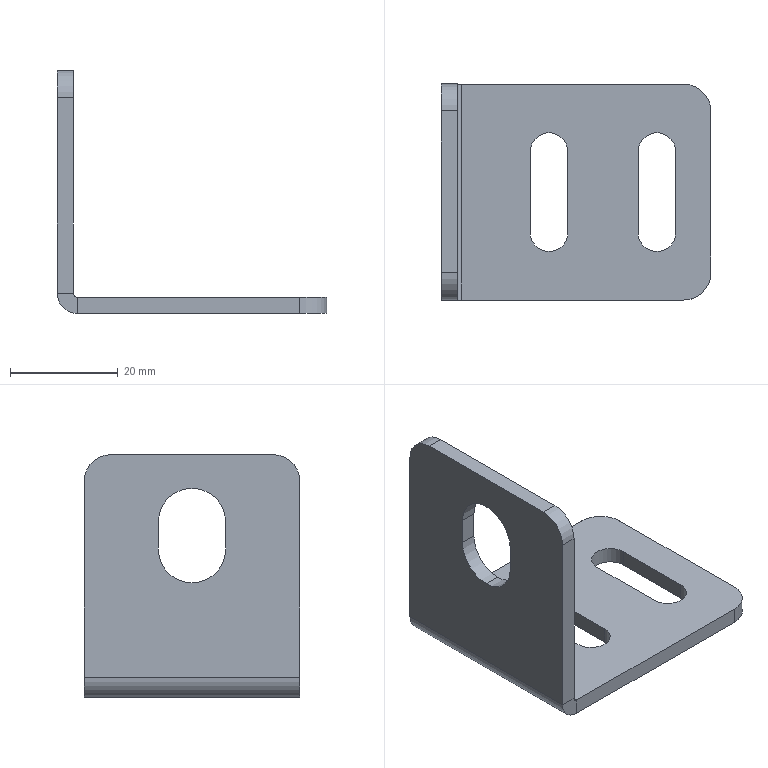Part | SolidWorks | features BaseBody 1 | 1 solid | 31 faces | box 50 x 40 x 45 mm | volume 9444 mm3 | plane 18 | cylinder 13 | commonest cylinder face diameters 7 x4 10 x4 12.5 x3 1.473 x1 7.473 x1
STEP:
#1=CARTESIAN_POINT('',(-25.,0.,18.25));
#2=VERTEX_POINT('',#1);
#3=CARTESIAN_POINT('',(-25.,6.25,24.5));
#4=VERTEX_POINT('',#3);
#5=CARTESIAN_POINT('',(-25.,0.,24.5));
#6=DIRECTION('',(1.,0.,0.));
#7=DIRECTION('',(0.,0.,-1.));
#8=AXIS2_PLACEMENT_3D('',#5,#6,#7);
#9=CIRCLE('',#8,6.25);
#10=EDGE_CURVE('',#2,#4,#9,.T.);
#11=ORIENTED_EDGE('',*,*,#10,.F.);
#12=CARTESIAN_POINT('',(-22.,0.,18.25));
#13=VERTEX_POINT('',#12);
#14=CARTESIAN_POINT('',(-32.,0.,18.25));
#15=DIRECTION('',(1.,0.,0.));
#16=VECTOR('',#15,1000.);
#17=LINE('',#14,#16);
#18=EDGE_CURVE('',#2,#13,#17,.T.);
#19=ORIENTED_EDGE('',*,*,#18,.T.);
#20=CARTESIAN_POINT('',(-22.,6.25,24.5));
#21=VERTEX_POINT('',#20);
#22=CARTESIAN_POINT('',(-22.,0.,24.5));
#23=DIRECTION('',(1.,0.,0.));
#24=DIRECTION('',(0.,0.,-1.));
#25=AXIS2_PLACEMENT_3D('',#22,#23,#24);
#26=CIRCLE('',#25,6.25);
#27=EDGE_CURVE('',#13,#21,#26,.T.);
#28=ORIENTED_EDGE('',*,*,#27,.T.);
#29=CARTESIAN_POINT('',(-32.,6.25,24.5));
#30=DIRECTION('',(1.,0.,0.));
#31=VECTOR('',#30,1000.);
#32=LINE('',#29,#31);
#33=EDGE_CURVE('',#4,#21,#32,.T.);
#34=ORIENTED_EDGE('',*,*,#33,.F.);
#35=EDGE_LOOP('',(#11,#19,#28,#34));
#36=FACE_OUTER_BOUND('',#35,.T.);
#37=CARTESIAN_POINT('',(-32.,0.,24.5));
#38=DIRECTION('',(1.,0.,0.));
#39=DIRECTION('',(0.,0.,-1.));
#40=AXIS2_PLACEMENT_3D('',#37,#38,#39);
#41=CYLINDRICAL_SURFACE('',#40,6.25);
#42=ADVANCED_FACE('',(#36),#41,.F.);
#43=CARTESIAN_POINT('',(-21.263,-20.,-3.));
#44=VERTEX_POINT('',#43);
#45=CARTESIAN_POINT('',(20.,-20.,-3.));
#46=VERTEX_POINT('',#45);
#47=CARTESIAN_POINT('',(-25.,-20.,-3.));
#48=DIRECTION('',(1.,0.,0.));
#49=VECTOR('',#48,1000.);
#50=LINE('',#47,#49);
#51=EDGE_CURVE('',#44,#46,#50,.T.);
#52=ORIENTED_EDGE('',*,*,#51,.T.);
#53=CARTESIAN_POINT('',(20.,-20.,0.));
#54=VERTEX_POINT('',#53);
#55=CARTESIAN_POINT('',(20.,-20.,-3.));
#56=DIRECTION('',(0.,0.,1.));
#57=VECTOR('',#56,1000.);
#58=LINE('',#55,#57);
#59=EDGE_CURVE('',#46,#54,#58,.T.);
#60=ORIENTED_EDGE('',*,*,#59,.T.);
#61=CARTESIAN_POINT('',(-21.263,-20.,0.));
#62=VERTEX_POINT('',#61);
#63=CARTESIAN_POINT('',(-25.,-20.,0.));
#64=DIRECTION('',(1.,0.,0.));
#65=VECTOR('',#64,1000.);
#66=LINE('',#63,#65);
#67=EDGE_CURVE('',#62,#54,#66,.T.);
#68=ORIENTED_EDGE('',*,*,#67,.F.);
#69=CARTESIAN_POINT('',(-21.263,-20.,0.));
#70=DIRECTION('',(0.,0.,-1.));
#71=VECTOR('',#70,1000.);
#72=LINE('',#69,#71);
#73=EDGE_CURVE('',#62,#44,#72,.T.);
#74=ORIENTED_EDGE('',*,*,#73,.T.);
#75=EDGE_LOOP('',(#52,#60,#68,#74));
#76=FACE_OUTER_BOUND('',#75,.T.);
#77=CARTESIAN_POINT('',(-25.,-20.,-3.));
#78=DIRECTION('',(0.,-1.,0.));
#79=DIRECTION('',(0.,0.,-1.));
#80=AXIS2_PLACEMENT_3D('',#77,#78,#79);
#81=PLANE('',#80);
#82=ADVANCED_FACE('',(#76),#81,.T.);
#83=CARTESIAN_POINT('',(18.5,-7.5,-3.));
#84=VERTEX_POINT('',#83);
#85=CARTESIAN_POINT('',(18.5,7.5,-3.));
#86=VERTEX_POINT('',#85);
#87=CARTESIAN_POINT('',(18.5,0.,-3.));
#88=DIRECTION('',(0.,1.,0.));
#89=VECTOR('',#88,1000.);
#90=LINE('',#87,#89);
#91=EDGE_CURVE('',#84,#86,#90,.T.);
#92=ORIENTED_EDGE('',*,*,#91,.T.);
#93=CARTESIAN_POINT('',(11.5,7.5,-3.));
#94=VERTEX_POINT('',#93);
#95=CARTESIAN_POINT('',(15.,7.5,-3.));
#96=DIRECTION('',(0.,0.,1.));
#97=DIRECTION('',(1.,0.,0.));
#98=AXIS2_PLACEMENT_3D('',#95,#96,#97);
#99=CIRCLE('',#98,3.5);
#100=EDGE_CURVE('',#86,#94,#99,.T.);
#101=ORIENTED_EDGE('',*,*,#100,.T.);
#102=CARTESIAN_POINT('',(11.5,-7.5,-3.));
#103=VERTEX_POINT('',#102);
#104=CARTESIAN_POINT('',(11.5,0.,-3.));
#105=DIRECTION('',(0.,-1.,0.));
#106=VECTOR('',#105,1000.);
#107=LINE('',#104,#106);
#108=EDGE_CURVE('',#94,#103,#107,.T.);
#109=ORIENTED_EDGE('',*,*,#108,.T.);
#110=CARTESIAN_POINT('',(15.,-7.5,-3.));
#111=DIRECTION('',(0.,0.,1.));
#112=DIRECTION('',(1.,0.,0.));
#113=AXIS2_PLACEMENT_3D('',#110,#111,#112);
#114=CIRCLE('',#113,3.5);
#115=EDGE_CURVE('',#103,#84,#114,.T.);
#116=ORIENTED_EDGE('',*,*,#115,.T.);
#117=EDGE_LOOP('',(#92,#101,#109,#116));
#118=FACE_BOUND('',#117,.T.);
#119=CARTESIAN_POINT('',(-1.5,-7.5,-3.));
#120=VERTEX_POINT('',#119);
#121=CARTESIAN_POINT('',(-1.5,7.5,-3.));
#122=VERTEX_POINT('',#121);
#123=CARTESIAN_POINT('',(-1.5,0.,-3.));
#124=DIRECTION('',(0.,1.,0.));
#125=VECTOR('',#124,1000.);
#126=LINE('',#123,#125);
#127=EDGE_CURVE('',#120,#122,#126,.T.);
#128=ORIENTED_EDGE('',*,*,#127,.T.);
#129=CARTESIAN_POINT('',(-8.5,7.5,-3.));
#130=VERTEX_POINT('',#129);
#131=CARTESIAN_POINT('',(-5.,7.5,-3.));
#132=DIRECTION('',(0.,0.,1.));
#133=DIRECTION('',(1.,0.,0.));
#134=AXIS2_PLACEMENT_3D('',#131,#132,#133);
#135=CIRCLE('',#134,3.5);
#136=EDGE_CURVE('',#122,#130,#135,.T.);
#137=ORIENTED_EDGE('',*,*,#136,.T.);
#138=CARTESIAN_POINT('',(-8.5,-7.5,-3.));
#139=VERTEX_POINT('',#138);
#140=CARTESIAN_POINT('',(-8.5,0.,-3.));
#141=DIRECTION('',(0.,-1.,0.));
#142=VECTOR('',#141,1000.);
#143=LINE('',#140,#142);
#144=EDGE_CURVE('',#130,#139,#143,.T.);
#145=ORIENTED_EDGE('',*,*,#144,.T.);
#146=CARTESIAN_POINT('',(-5.,-7.5,-3.));
#147=DIRECTION('',(0.,0.,1.));
#148=DIRECTION('',(1.,0.,0.));
#149=AXIS2_PLACEMENT_3D('',#146,#147,#148);
#150=CIRCLE('',#149,3.5);
#151=EDGE_CURVE('',#139,#120,#150,.T.);
#152=ORIENTED_EDGE('',*,*,#151,.T.);
#153=EDGE_LOOP('',(#128,#137,#145,#152));
#154=FACE_BOUND('',#153,.T.);
#155=CARTESIAN_POINT('',(20.,20.,-3.));
#156=VERTEX_POINT('',#155);
#157=CARTESIAN_POINT('',(-21.263,20.,-3.));
#158=VERTEX_POINT('',#157);
#159=CARTESIAN_POINT('',(-25.,20.,-3.));
#160=DIRECTION('',(-1.,0.,0.));
#161=VECTOR('',#160,1000.);
#162=LINE('',#159,#161);
#163=EDGE_CURVE('',#156,#158,#162,.T.);
#164=ORIENTED_EDGE('',*,*,#163,.F.);
#165=CARTESIAN_POINT('',(25.,15.,-3.));
#166=VERTEX_POINT('',#165);
#167=CARTESIAN_POINT('',(20.,15.,-3.));
#168=DIRECTION('',(0.,0.,-1.));
#169=DIRECTION('',(1.,0.,0.));
#170=AXIS2_PLACEMENT_3D('',#167,#168,#169);
#171=CIRCLE('',#170,5.);
#172=EDGE_CURVE('',#156,#166,#171,.T.);
#173=ORIENTED_EDGE('',*,*,#172,.T.);
#174=CARTESIAN_POINT('',(25.,-15.,-3.));
#175=VERTEX_POINT('',#174);
#176=CARTESIAN_POINT('',(25.,20.,-3.));
#177=DIRECTION('',(0.,1.,0.));
#178=VECTOR('',#177,1000.);
#179=LINE('',#176,#178);
#180=EDGE_CURVE('',#175,#166,#179,.T.);
#181=ORIENTED_EDGE('',*,*,#180,.F.);
#182=CARTESIAN_POINT('',(20.,-15.,-3.));
#183=DIRECTION('',(0.,0.,-1.));
#184=DIRECTION('',(1.,0.,0.));
#185=AXIS2_PLACEMENT_3D('',#182,#183,#184);
#186=CIRCLE('',#185,5.);
#187=EDGE_CURVE('',#175,#46,#186,.T.);
#188=ORIENTED_EDGE('',*,*,#187,.T.);
#189=ORIENTED_EDGE('',*,*,#51,.F.);
#190=CARTESIAN_POINT('',(-21.263,-20.,-3.));
#191=DIRECTION('',(0.,1.,0.));
#192=VECTOR('',#191,1000.);
#193=LINE('',#190,#192);
#194=EDGE_CURVE('',#44,#158,#193,.T.);
#195=ORIENTED_EDGE('',*,*,#194,.T.);
#196=EDGE_LOOP('',(#164,#173,#181,#188,#189,#195));
#197=FACE_OUTER_BOUND('',#196,.T.);
#198=CARTESIAN_POINT('',(0.,0.,-3.));
#199=DIRECTION('',(0.,0.,1.));
#200=DIRECTION('',(1.,0.,0.));
#201=AXIS2_PLACEMENT_3D('',#198,#199,#200);
#202=PLANE('',#201);
#203=ADVANCED_FACE('',(#118,#154,#197),#202,.F.);
#204=CARTESIAN_POINT('',(18.5,7.5,0.));
#205=VERTEX_POINT('',#204);
#206=CARTESIAN_POINT('',(11.5,7.5,0.));
#207=VERTEX_POINT('',#206);
#208=CARTESIAN_POINT('',(15.,7.5,0.));
#209=DIRECTION('',(0.,0.,1.));
#210=DIRECTION('',(1.,0.,0.));
#211=AXIS2_PLACEMENT_3D('',#208,#209,#210);
#212=CIRCLE('',#211,3.5);
#213=EDGE_CURVE('',#205,#207,#212,.T.);
#214=ORIENTED_EDGE('',*,*,#213,.F.);
#215=CARTESIAN_POINT('',(18.5,-7.5,0.));
#216=VERTEX_POINT('',#215);
#217=CARTESIAN_POINT('',(18.5,7.5,0.));
#218=DIRECTION('',(0.,1.,0.));
#219=VECTOR('',#218,1000.);
#220=LINE('',#217,#219);
#221=EDGE_CURVE('',#216,#205,#220,.T.);
#222=ORIENTED_EDGE('',*,*,#221,.F.);
#223=CARTESIAN_POINT('',(11.5,-7.5,0.));
#224=VERTEX_POINT('',#223);
#225=CARTESIAN_POINT('',(15.,-7.5,0.));
#226=DIRECTION('',(0.,0.,1.));
#227=DIRECTION('',(1.,0.,0.));
#228=AXIS2_PLACEMENT_3D('',#225,#226,#227);
#229=CIRCLE('',#228,3.5);
#230=EDGE_CURVE('',#224,#216,#229,.T.);
#231=ORIENTED_EDGE('',*,*,#230,.F.);
#232=CARTESIAN_POINT('',(11.5,7.5,0.));
#233=DIRECTION('',(0.,-1.,0.));
#234=VECTOR('',#233,1000.);
#235=LINE('',#232,#234);
#236=EDGE_CURVE('',#207,#224,#235,.T.);
#237=ORIENTED_EDGE('',*,*,#236,.F.);
#238=EDGE_LOOP('',(#214,#222,#231,#237));
#239=FACE_BOUND('',#238,.T.);
#240=CARTESIAN_POINT('',(-1.5,7.5,0.));
#241=VERTEX_POINT('',#240);
#242=CARTESIAN_POINT('',(-8.5,7.5,0.));
#243=VERTEX_POINT('',#242);
#244=CARTESIAN_POINT('',(-5.,7.5,0.));
#245=DIRECTION('',(0.,0.,1.));
#246=DIRECTION('',(1.,0.,0.));
#247=AXIS2_PLACEMENT_3D('',#244,#245,#246);
#248=CIRCLE('',#247,3.5);
#249=EDGE_CURVE('',#241,#243,#248,.T.);
#250=ORIENTED_EDGE('',*,*,#249,.F.);
#251=CARTESIAN_POINT('',(-1.5,-7.5,0.));
#252=VERTEX_POINT('',#251);
#253=CARTESIAN_POINT('',(-1.5,7.5,0.));
#254=DIRECTION('',(0.,1.,0.));
#255=VECTOR('',#254,1000.);
#256=LINE('',#253,#255);
#257=EDGE_CURVE('',#252,#241,#256,.T.);
#258=ORIENTED_EDGE('',*,*,#257,.F.);
#259=CARTESIAN_POINT('',(-8.5,-7.5,0.));
#260=VERTEX_POINT('',#259);
#261=CARTESIAN_POINT('',(-5.,-7.5,0.));
#262=DIRECTION('',(0.,0.,1.));
#263=DIRECTION('',(1.,0.,0.));
#264=AXIS2_PLACEMENT_3D('',#261,#262,#263);
#265=CIRCLE('',#264,3.5);
#266=EDGE_CURVE('',#260,#252,#265,.T.);
#267=ORIENTED_EDGE('',*,*,#266,.F.);
#268=CARTESIAN_POINT('',(-8.5,7.5,0.));
#269=DIRECTION('',(0.,-1.,0.));
#270=VECTOR('',#269,1000.);
#271=LINE('',#268,#270);
#272=EDGE_CURVE('',#243,#260,#271,.T.);
#273=ORIENTED_EDGE('',*,*,#272,.F.);
#274=EDGE_LOOP('',(#250,#258,#267,#273));
#275=FACE_BOUND('',#274,.T.);
#276=CARTESIAN_POINT('',(25.,-15.,0.));
#277=VERTEX_POINT('',#276);
#278=CARTESIAN_POINT('',(25.,15.,0.));
#279=VERTEX_POINT('',#278);
#280=CARTESIAN_POINT('',(25.,20.,0.));
#281=DIRECTION('',(0.,1.,0.));
#282=VECTOR('',#281,1000.);
#283=LINE('',#280,#282);
#284=EDGE_CURVE('',#277,#279,#283,.T.);
#285=ORIENTED_EDGE('',*,*,#284,.T.);
#286=CARTESIAN_POINT('',(20.,20.,0.));
#287=VERTEX_POINT('',#286);
#288=CARTESIAN_POINT('',(20.,15.,0.));
#289=DIRECTION('',(0.,0.,1.));
#290=DIRECTION('',(1.,0.,0.));
#291=AXIS2_PLACEMENT_3D('',#288,#289,#290);
#292=CIRCLE('',#291,5.);
#293=EDGE_CURVE('',#279,#287,#292,.T.);
#294=ORIENTED_EDGE('',*,*,#293,.T.);
#295=CARTESIAN_POINT('',(-21.263,20.,0.));
#296=VERTEX_POINT('',#295);
#297=CARTESIAN_POINT('',(-25.,20.,0.));
#298=DIRECTION('',(-1.,0.,0.));
#299=VECTOR('',#298,1000.);
#300=LINE('',#297,#299);
#301=EDGE_CURVE('',#287,#296,#300,.T.);
#302=ORIENTED_EDGE('',*,*,#301,.T.);
#303=CARTESIAN_POINT('',(-21.263,-20.,0.));
#304=DIRECTION('',(0.,1.,0.));
#305=VECTOR('',#304,1000.);
#306=LINE('',#303,#305);
#307=EDGE_CURVE('',#62,#296,#306,.T.);
#308=ORIENTED_EDGE('',*,*,#307,.F.);
#309=ORIENTED_EDGE('',*,*,#67,.T.);
#310=CARTESIAN_POINT('',(20.,-15.,0.));
#311=DIRECTION('',(0.,0.,1.));
#312=DIRECTION('',(1.,0.,0.));
#313=AXIS2_PLACEMENT_3D('',#310,#311,#312);
#314=CIRCLE('',#313,5.);
#315=EDGE_CURVE('',#54,#277,#314,.T.);
#316=ORIENTED_EDGE('',*,*,#315,.T.);
#317=EDGE_LOOP('',(#285,#294,#302,#308,#309,#316));
#318=FACE_OUTER_BOUND('',#317,.T.);
#319=CARTESIAN_POINT('',(0.,0.,0.));
#320=DIRECTION('',(0.,0.,1.));
#321=DIRECTION('',(1.,0.,0.));
#322=AXIS2_PLACEMENT_3D('',#319,#320,#321);
#323=PLANE('',#322);
#324=ADVANCED_FACE('',(#239,#275,#318),#323,.T.);
#325=ORIENTED_EDGE('',*,*,#180,.T.);
#326=CARTESIAN_POINT('',(25.,15.,-3.));
#327=DIRECTION('',(0.,0.,1.));
#328=VECTOR('',#327,1000.);
#329=LINE('',#326,#328);
#330=EDGE_CURVE('',#166,#279,#329,.T.);
#331=ORIENTED_EDGE('',*,*,#330,.T.);
#332=ORIENTED_EDGE('',*,*,#284,.F.);
#333=CARTESIAN_POINT('',(25.,-15.,-3.));
#334=DIRECTION('',(0.,0.,-1.));
#335=VECTOR('',#334,1000.);
#336=LINE('',#333,#335);
#337=EDGE_CURVE('',#277,#175,#336,.T.);
#338=ORIENTED_EDGE('',*,*,#337,.T.);
#339=EDGE_LOOP('',(#325,#331,#332,#338));
#340=FACE_OUTER_BOUND('',#339,.T.);
#341=CARTESIAN_POINT('',(25.,20.,-3.));
#342=DIRECTION('',(1.,0.,0.));
#343=DIRECTION('',(0.,0.,-1.));
#344=AXIS2_PLACEMENT_3D('',#341,#342,#343);
#345=PLANE('',#344);
#346=ADVANCED_FACE('',(#340),#345,.T.);
#347=ORIENTED_EDGE('',*,*,#301,.F.);
#348=CARTESIAN_POINT('',(20.,20.,-3.));
#349=DIRECTION('',(0.,0.,-1.));
#350=VECTOR('',#349,1000.);
#351=LINE('',#348,#350);
#352=EDGE_CURVE('',#287,#156,#351,.T.);
#353=ORIENTED_EDGE('',*,*,#352,.T.);
#354=ORIENTED_EDGE('',*,*,#163,.T.);
#355=CARTESIAN_POINT('',(-21.263,20.,0.));
#356=DIRECTION('',(0.,0.,-1.));
#357=VECTOR('',#356,1000.);
#358=LINE('',#355,#357);
#359=EDGE_CURVE('',#296,#158,#358,.T.);
#360=ORIENTED_EDGE('',*,*,#359,.F.);
#361=EDGE_LOOP('',(#347,#353,#354,#360));
#362=FACE_OUTER_BOUND('',#361,.T.);
#363=CARTESIAN_POINT('',(-25.,20.,-3.));
#364=DIRECTION('',(0.,1.,0.));
#365=DIRECTION('',(0.,0.,1.));
#366=AXIS2_PLACEMENT_3D('',#363,#364,#365);
#367=PLANE('',#366);
#368=ADVANCED_FACE('',(#362),#367,.T.);
#369=CARTESIAN_POINT('',(-22.,20.,0.7366));
#370=VERTEX_POINT('',#369);
#371=CARTESIAN_POINT('',(-25.,20.,0.7366));
#372=VERTEX_POINT('',#371);
#373=CARTESIAN_POINT('',(-25.,20.,0.7366));
#374=DIRECTION('',(-1.,0.,0.));
#375=VECTOR('',#374,1000.);
#376=LINE('',#373,#375);
#377=EDGE_CURVE('',#370,#372,#376,.T.);
#378=ORIENTED_EDGE('',*,*,#377,.F.);
#379=CARTESIAN_POINT('',(-21.263,20.,0.7366));
#380=DIRECTION('',(0.,1.,0.));
#381=DIRECTION('',(0.,0.,-1.));
#382=AXIS2_PLACEMENT_3D('',#379,#380,#381);
#383=CIRCLE('',#382,0.7366);
#384=EDGE_CURVE('',#296,#370,#383,.T.);
#385=ORIENTED_EDGE('',*,*,#384,.F.);
#386=ORIENTED_EDGE('',*,*,#359,.T.);
#387=CARTESIAN_POINT('',(-21.263,20.,0.7366));
#388=DIRECTION('',(0.,1.,0.));
#389=DIRECTION('',(0.,0.,-1.));
#390=AXIS2_PLACEMENT_3D('',#387,#388,#389);
#391=CIRCLE('',#390,3.737);
#392=EDGE_CURVE('',#158,#372,#391,.T.);
#393=ORIENTED_EDGE('',*,*,#392,.T.);
#394=EDGE_LOOP('',(#378,#385,#386,#393));
#395=FACE_OUTER_BOUND('',#394,.T.);
#396=CARTESIAN_POINT('',(-21.263,20.,0.7366));
#397=DIRECTION('',(0.,1.,0.));
#398=DIRECTION('',(0.,0.,1.));
#399=AXIS2_PLACEMENT_3D('',#396,#397,#398);
#400=PLANE('',#399);
#401=ADVANCED_FACE('',(#395),#400,.T.);
#402=CARTESIAN_POINT('',(-22.,-20.,0.7366));
#403=VERTEX_POINT('',#402);
#404=CARTESIAN_POINT('',(-21.263,-20.,0.7366));
#405=DIRECTION('',(0.,-1.,0.));
#406=DIRECTION('',(0.,0.,-1.));
#407=AXIS2_PLACEMENT_3D('',#404,#405,#406);
#408=CIRCLE('',#407,0.7366);
#409=EDGE_CURVE('',#403,#62,#408,.T.);
#410=ORIENTED_EDGE('',*,*,#409,.F.);
#411=CARTESIAN_POINT('',(-25.,-20.,0.7366));
#412=VERTEX_POINT('',#411);
#413=CARTESIAN_POINT('',(-22.,-20.,0.7366));
#414=DIRECTION('',(-1.,0.,0.));
#415=VECTOR('',#414,1000.);
#416=LINE('',#413,#415);
#417=EDGE_CURVE('',#403,#412,#416,.T.);
#418=ORIENTED_EDGE('',*,*,#417,.T.);
#419=CARTESIAN_POINT('',(-21.263,-20.,0.7366));
#420=DIRECTION('',(0.,-1.,0.));
#421=DIRECTION('',(0.,0.,-1.));
#422=AXIS2_PLACEMENT_3D('',#419,#420,#421);
#423=CIRCLE('',#422,3.737);
#424=EDGE_CURVE('',#412,#44,#423,.T.);
#425=ORIENTED_EDGE('',*,*,#424,.T.);
#426=ORIENTED_EDGE('',*,*,#73,.F.);
#427=EDGE_LOOP('',(#410,#418,#425,#426));
#428=FACE_OUTER_BOUND('',#427,.T.);
#429=CARTESIAN_POINT('',(-21.263,-20.,0.7366));
#430=DIRECTION('',(0.,1.,0.));
#431=DIRECTION('',(0.,0.,1.));
#432=AXIS2_PLACEMENT_3D('',#429,#430,#431);
#433=PLANE('',#432);
#434=ADVANCED_FACE('',(#428),#433,.F.);
#435=ORIENTED_EDGE('',*,*,#194,.F.);
#436=ORIENTED_EDGE('',*,*,#424,.F.);
#437=CARTESIAN_POINT('',(-25.,20.,0.7366));
#438=DIRECTION('',(0.,1.,0.));
#439=VECTOR('',#438,1000.);
#440=LINE('',#437,#439);
#441=EDGE_CURVE('',#412,#372,#440,.T.);
#442=ORIENTED_EDGE('',*,*,#441,.T.);
#443=ORIENTED_EDGE('',*,*,#392,.F.);
#444=EDGE_LOOP('',(#435,#436,#442,#443));
#445=FACE_OUTER_BOUND('',#444,.T.);
#446=CARTESIAN_POINT('',(-21.263,-20.,0.7366));
#447=DIRECTION('',(0.,-1.,0.));
#448=DIRECTION('',(-1.,0.,0.));
#449=AXIS2_PLACEMENT_3D('',#446,#447,#448);
#450=CYLINDRICAL_SURFACE('',#449,3.737);
#451=ADVANCED_FACE('',(#445),#450,.T.);
#452=ORIENTED_EDGE('',*,*,#307,.T.);
#453=ORIENTED_EDGE('',*,*,#384,.T.);
#454=CARTESIAN_POINT('',(-22.,20.,0.7366));
#455=DIRECTION('',(0.,-1.,0.));
#456=VECTOR('',#455,1000.);
#457=LINE('',#454,#456);
#458=EDGE_CURVE('',#370,#403,#457,.T.);
#459=ORIENTED_EDGE('',*,*,#458,.T.);
#460=ORIENTED_EDGE('',*,*,#409,.T.);
#461=EDGE_LOOP('',(#452,#453,#459,#460));
#462=FACE_OUTER_BOUND('',#461,.T.);
#463=CARTESIAN_POINT('',(-21.263,-20.,0.7366));
#464=DIRECTION('',(0.,-1.,0.));
#465=DIRECTION('',(-1.,0.,0.));
#466=AXIS2_PLACEMENT_3D('',#463,#464,#465);
#467=CYLINDRICAL_SURFACE('',#466,0.7366);
#468=ADVANCED_FACE('',(#462),#467,.F.);
#469=CARTESIAN_POINT('',(-25.,20.,37.));
#470=VERTEX_POINT('',#469);
#471=CARTESIAN_POINT('',(-25.,20.,0.));
#472=DIRECTION('',(0.,0.,-1.));
#473=VECTOR('',#472,1000.);
#474=LINE('',#471,#473);
#475=EDGE_CURVE('',#470,#372,#474,.T.);
#476=ORIENTED_EDGE('',*,*,#475,.F.);
#477=CARTESIAN_POINT('',(-22.,20.,37.));
#478=VERTEX_POINT('',#477);
#479=CARTESIAN_POINT('',(-25.,20.,37.));
#480=DIRECTION('',(1.,0.,0.));
#481=VECTOR('',#480,1000.);
#482=LINE('',#479,#481);
#483=EDGE_CURVE('',#470,#478,#482,.T.);
#484=ORIENTED_EDGE('',*,*,#483,.T.);
#485=CARTESIAN_POINT('',(-22.,20.,0.));
#486=DIRECTION('',(0.,0.,-1.));
#487=VECTOR('',#486,1000.);
#488=LINE('',#485,#487);
#489=EDGE_CURVE('',#478,#370,#488,.T.);
#490=ORIENTED_EDGE('',*,*,#489,.T.);
#491=ORIENTED_EDGE('',*,*,#377,.T.);
#492=EDGE_LOOP('',(#476,#484,#490,#491));
#493=FACE_OUTER_BOUND('',#492,.T.);
#494=CARTESIAN_POINT('',(-25.,20.,0.));
#495=DIRECTION('',(0.,-1.,0.));
#496=DIRECTION('',(1.,0.,0.));
#497=AXIS2_PLACEMENT_3D('',#494,#495,#496);
#498=PLANE('',#497);
#499=ADVANCED_FACE('',(#493),#498,.F.);
#500=CARTESIAN_POINT('',(-22.,-20.,37.));
#501=VERTEX_POINT('',#500);
#502=CARTESIAN_POINT('',(-22.,-20.,42.));
#503=DIRECTION('',(0.,0.,1.));
#504=VECTOR('',#503,1000.);
#505=LINE('',#502,#504);
#506=EDGE_CURVE('',#403,#501,#505,.T.);
#507=ORIENTED_EDGE('',*,*,#506,.T.);
#508=CARTESIAN_POINT('',(-25.,-20.,37.));
#509=VERTEX_POINT('',#508);
#510=CARTESIAN_POINT('',(-25.,-20.,37.));
#511=DIRECTION('',(-1.,0.,0.));
#512=VECTOR('',#511,1000.);
#513=LINE('',#510,#512);
#514=EDGE_CURVE('',#501,#509,#513,.T.);
#515=ORIENTED_EDGE('',*,*,#514,.T.);
#516=CARTESIAN_POINT('',(-25.,-20.,0.));
#517=DIRECTION('',(0.,0.,1.));
#518=VECTOR('',#517,1000.);
#519=LINE('',#516,#518);
#520=EDGE_CURVE('',#412,#509,#519,.T.);
#521=ORIENTED_EDGE('',*,*,#520,.F.);
#522=ORIENTED_EDGE('',*,*,#417,.F.);
#523=EDGE_LOOP('',(#507,#515,#521,#522));
#524=FACE_OUTER_BOUND('',#523,.T.);
#525=CARTESIAN_POINT('',(-25.,-20.,42.));
#526=DIRECTION('',(0.,1.,0.));
#527=DIRECTION('',(-1.,0.,0.));
#528=AXIS2_PLACEMENT_3D('',#525,#526,#527);
#529=PLANE('',#528);
#530=ADVANCED_FACE('',(#524),#529,.F.);
#531=CARTESIAN_POINT('',(-25.,6.25,29.5));
#532=VERTEX_POINT('',#531);
#533=CARTESIAN_POINT('',(-25.,6.25,0.));
#534=DIRECTION('',(0.,0.,1.));
#535=VECTOR('',#534,1000.);
#536=LINE('',#533,#535);
#537=EDGE_CURVE('',#4,#532,#536,.T.);
#538=ORIENTED_EDGE('',*,*,#537,.T.);
#539=CARTESIAN_POINT('',(-25.,-6.25,29.5));
#540=VERTEX_POINT('',#539);
#541=CARTESIAN_POINT('',(-25.,0.,29.5));
#542=DIRECTION('',(1.,0.,0.));
#543=DIRECTION('',(0.,0.,-1.));
#544=AXIS2_PLACEMENT_3D('',#541,#542,#543);
#545=CIRCLE('',#544,6.25);
#546=EDGE_CURVE('',#532,#540,#545,.T.);
#547=ORIENTED_EDGE('',*,*,#546,.T.);
#548=CARTESIAN_POINT('',(-25.,-6.25,24.5));
#549=VERTEX_POINT('',#548);
#550=CARTESIAN_POINT('',(-25.,-6.25,0.));
#551=DIRECTION('',(0.,0.,-1.));
#552=VECTOR('',#551,1000.);
#553=LINE('',#550,#552);
#554=EDGE_CURVE('',#540,#549,#553,.T.);
#555=ORIENTED_EDGE('',*,*,#554,.T.);
#556=CARTESIAN_POINT('',(-25.,0.,24.5));
#557=DIRECTION('',(1.,0.,0.));
#558=DIRECTION('',(0.,0.,-1.));
#559=AXIS2_PLACEMENT_3D('',#556,#557,#558);
#560=CIRCLE('',#559,6.25);
#561=EDGE_CURVE('',#549,#2,#560,.T.);
#562=ORIENTED_EDGE('',*,*,#561,.T.);
#563=ORIENTED_EDGE('',*,*,#10,.T.);
#564=EDGE_LOOP('',(#538,#547,#555,#562,#563));
#565=FACE_BOUND('',#564,.T.);
#566=ORIENTED_EDGE('',*,*,#520,.T.);
#567=CARTESIAN_POINT('',(-25.,-15.,42.));
#568=VERTEX_POINT('',#567);
#569=CARTESIAN_POINT('',(-25.,-15.,37.));
#570=DIRECTION('',(-1.,0.,0.));
#571=DIRECTION('',(0.,0.,-1.));
#572=AXIS2_PLACEMENT_3D('',#569,#570,#571);
#573=CIRCLE('',#572,5.);
#574=EDGE_CURVE('',#509,#568,#573,.T.);
#575=ORIENTED_EDGE('',*,*,#574,.T.);
#576=CARTESIAN_POINT('',(-25.,15.,42.));
#577=VERTEX_POINT('',#576);
#578=CARTESIAN_POINT('',(-25.,0.,42.));
#579=DIRECTION('',(0.,1.,0.));
#580=VECTOR('',#579,1000.);
#581=LINE('',#578,#580);
#582=EDGE_CURVE('',#568,#577,#581,.T.);
#583=ORIENTED_EDGE('',*,*,#582,.T.);
#584=CARTESIAN_POINT('',(-25.,15.,37.));
#585=DIRECTION('',(-1.,0.,0.));
#586=DIRECTION('',(0.,0.,-1.));
#587=AXIS2_PLACEMENT_3D('',#584,#585,#586);
#588=CIRCLE('',#587,5.);
#589=EDGE_CURVE('',#577,#470,#588,.T.);
#590=ORIENTED_EDGE('',*,*,#589,.T.);
#591=ORIENTED_EDGE('',*,*,#475,.T.);
#592=ORIENTED_EDGE('',*,*,#441,.F.);
#593=EDGE_LOOP('',(#566,#575,#583,#590,#591,#592));
#594=FACE_OUTER_BOUND('',#593,.T.);
#595=CARTESIAN_POINT('',(-25.,0.,0.));
#596=DIRECTION('',(1.,0.,0.));
#597=DIRECTION('',(0.,0.,-1.));
#598=AXIS2_PLACEMENT_3D('',#595,#596,#597);
#599=PLANE('',#598);
#600=ADVANCED_FACE('',(#565,#594),#599,.F.);
#601=CARTESIAN_POINT('',(-22.,6.25,29.5));
#602=VERTEX_POINT('',#601);
#603=CARTESIAN_POINT('',(-22.,-6.25,29.5));
#604=VERTEX_POINT('',#603);
#605=CARTESIAN_POINT('',(-22.,0.,29.5));
#606=DIRECTION('',(1.,0.,0.));
#607=DIRECTION('',(0.,0.,-1.));
#608=AXIS2_PLACEMENT_3D('',#605,#606,#607);
#609=CIRCLE('',#608,6.25);
#610=EDGE_CURVE('',#602,#604,#609,.T.);
#611=ORIENTED_EDGE('',*,*,#610,.F.);
#612=CARTESIAN_POINT('',(-22.,6.25,29.5));
#613=DIRECTION('',(0.,0.,1.));
#614=VECTOR('',#613,1000.);
#615=LINE('',#612,#614);
#616=EDGE_CURVE('',#21,#602,#615,.T.);
#617=ORIENTED_EDGE('',*,*,#616,.F.);
#618=ORIENTED_EDGE('',*,*,#27,.F.);
#619=CARTESIAN_POINT('',(-22.,-6.25,24.5));
#620=VERTEX_POINT('',#619);
#621=CARTESIAN_POINT('',(-22.,0.,24.5));
#622=DIRECTION('',(1.,0.,0.));
#623=DIRECTION('',(0.,0.,-1.));
#624=AXIS2_PLACEMENT_3D('',#621,#622,#623);
#625=CIRCLE('',#624,6.25);
#626=EDGE_CURVE('',#620,#13,#625,.T.);
#627=ORIENTED_EDGE('',*,*,#626,.F.);
#628=CARTESIAN_POINT('',(-22.,-6.25,29.5));
#629=DIRECTION('',(0.,0.,-1.));
#630=VECTOR('',#629,1000.);
#631=LINE('',#628,#630);
#632=EDGE_CURVE('',#604,#620,#631,.T.);
#633=ORIENTED_EDGE('',*,*,#632,.F.);
#634=EDGE_LOOP('',(#611,#617,#618,#627,#633));
#635=FACE_BOUND('',#634,.T.);
#636=CARTESIAN_POINT('',(-22.,-15.,42.));
#637=VERTEX_POINT('',#636);
#638=CARTESIAN_POINT('',(-22.,15.,42.));
#639=VERTEX_POINT('',#638);
#640=CARTESIAN_POINT('',(-22.,20.,42.));
#641=DIRECTION('',(0.,1.,0.));
#642=VECTOR('',#641,1000.);
#643=LINE('',#640,#642);
#644=EDGE_CURVE('',#637,#639,#643,.T.);
#645=ORIENTED_EDGE('',*,*,#644,.F.);
#646=CARTESIAN_POINT('',(-22.,-15.,37.));
#647=DIRECTION('',(1.,0.,0.));
#648=DIRECTION('',(0.,0.,-1.));
#649=AXIS2_PLACEMENT_3D('',#646,#647,#648);
#650=CIRCLE('',#649,5.);
#651=EDGE_CURVE('',#637,#501,#650,.T.);
#652=ORIENTED_EDGE('',*,*,#651,.T.);
#653=ORIENTED_EDGE('',*,*,#506,.F.);
#654=ORIENTED_EDGE('',*,*,#458,.F.);
#655=ORIENTED_EDGE('',*,*,#489,.F.);
#656=CARTESIAN_POINT('',(-22.,15.,37.));
#657=DIRECTION('',(1.,0.,0.));
#658=DIRECTION('',(0.,0.,-1.));
#659=AXIS2_PLACEMENT_3D('',#656,#657,#658);
#660=CIRCLE('',#659,5.);
#661=EDGE_CURVE('',#478,#639,#660,.T.);
#662=ORIENTED_EDGE('',*,*,#661,.T.);
#663=EDGE_LOOP('',(#645,#652,#653,#654,#655,#662));
#664=FACE_OUTER_BOUND('',#663,.T.);
#665=CARTESIAN_POINT('',(-22.,0.,0.));
#666=DIRECTION('',(1.,0.,0.));
#667=DIRECTION('',(0.,0.,-1.));
#668=AXIS2_PLACEMENT_3D('',#665,#666,#667);
#669=PLANE('',#668);
#670=ADVANCED_FACE('',(#635,#664),#669,.T.);
#671=ORIENTED_EDGE('',*,*,#582,.F.);
#672=CARTESIAN_POINT('',(-25.,-15.,42.));
#673=DIRECTION('',(1.,0.,0.));
#674=VECTOR('',#673,1000.);
#675=LINE('',#672,#674);
#676=EDGE_CURVE('',#568,#637,#675,.T.);
#677=ORIENTED_EDGE('',*,*,#676,.T.);
#678=ORIENTED_EDGE('',*,*,#644,.T.);
#679=CARTESIAN_POINT('',(-25.,15.,42.));
#680=DIRECTION('',(-1.,0.,0.));
#681=VECTOR('',#680,1000.);
#682=LINE('',#679,#681);
#683=EDGE_CURVE('',#639,#577,#682,.T.);
#684=ORIENTED_EDGE('',*,*,#683,.T.);
#685=EDGE_LOOP('',(#671,#677,#678,#684));
#686=FACE_OUTER_BOUND('',#685,.T.);
#687=CARTESIAN_POINT('',(-25.,20.,42.));
#688=DIRECTION('',(0.,0.,-1.));
#689=DIRECTION('',(-1.,0.,0.));
#690=AXIS2_PLACEMENT_3D('',#687,#688,#689);
#691=PLANE('',#690);
#692=ADVANCED_FACE('',(#686),#691,.F.);
#693=CARTESIAN_POINT('',(-1.5,7.5,-10.));
#694=DIRECTION('',(0.,0.,1.));
#695=VECTOR('',#694,1000.);
#696=LINE('',#693,#695);
#697=EDGE_CURVE('',#122,#241,#696,.T.);
#698=ORIENTED_EDGE('',*,*,#697,.T.);
#699=ORIENTED_EDGE('',*,*,#249,.T.);
#700=CARTESIAN_POINT('',(-8.5,7.5,-10.));
#701=DIRECTION('',(0.,0.,1.));
#702=VECTOR('',#701,1000.);
#703=LINE('',#700,#702);
#704=EDGE_CURVE('',#130,#243,#703,.T.);
#705=ORIENTED_EDGE('',*,*,#704,.F.);
#706=ORIENTED_EDGE('',*,*,#136,.F.);
#707=EDGE_LOOP('',(#698,#699,#705,#706));
#708=FACE_OUTER_BOUND('',#707,.T.);
#709=CARTESIAN_POINT('',(-5.,7.5,-10.));
#710=DIRECTION('',(0.,0.,1.));
#711=DIRECTION('',(1.,0.,0.));
#712=AXIS2_PLACEMENT_3D('',#709,#710,#711);
#713=CYLINDRICAL_SURFACE('',#712,3.5);
#714=ADVANCED_FACE('',(#708),#713,.F.);
#715=CARTESIAN_POINT('',(-1.5,-7.5,-10.));
#716=DIRECTION('',(0.,0.,1.));
#717=VECTOR('',#716,1000.);
#718=LINE('',#715,#717);
#719=EDGE_CURVE('',#120,#252,#718,.T.);
#720=ORIENTED_EDGE('',*,*,#719,.T.);
#721=ORIENTED_EDGE('',*,*,#257,.T.);
#722=ORIENTED_EDGE('',*,*,#697,.F.);
#723=ORIENTED_EDGE('',*,*,#127,.F.);
#724=EDGE_LOOP('',(#720,#721,#722,#723));
#725=FACE_OUTER_BOUND('',#724,.T.);
#726=CARTESIAN_POINT('',(-1.5,7.5,-10.));
#727=DIRECTION('',(1.,0.,0.));
#728=DIRECTION('',(0.,1.,0.));
#729=AXIS2_PLACEMENT_3D('',#726,#727,#728);
#730=PLANE('',#729);
#731=ADVANCED_FACE('',(#725),#730,.F.);
#732=CARTESIAN_POINT('',(-8.5,-7.5,-10.));
#733=DIRECTION('',(0.,0.,1.));
#734=VECTOR('',#733,1000.);
#735=LINE('',#732,#734);
#736=EDGE_CURVE('',#139,#260,#735,.T.);
#737=ORIENTED_EDGE('',*,*,#736,.T.);
#738=ORIENTED_EDGE('',*,*,#266,.T.);
#739=ORIENTED_EDGE('',*,*,#719,.F.);
#740=ORIENTED_EDGE('',*,*,#151,.F.);
#741=EDGE_LOOP('',(#737,#738,#739,#740));
#742=FACE_OUTER_BOUND('',#741,.T.);
#743=CARTESIAN_POINT('',(-5.,-7.5,-10.));
#744=DIRECTION('',(0.,0.,1.));
#745=DIRECTION('',(1.,0.,0.));
#746=AXIS2_PLACEMENT_3D('',#743,#744,#745);
#747=CYLINDRICAL_SURFACE('',#746,3.5);
#748=ADVANCED_FACE('',(#742),#747,.F.);
#749=ORIENTED_EDGE('',*,*,#704,.T.);
#750=ORIENTED_EDGE('',*,*,#272,.T.);
#751=ORIENTED_EDGE('',*,*,#736,.F.);
#752=ORIENTED_EDGE('',*,*,#144,.F.);
#753=EDGE_LOOP('',(#749,#750,#751,#752));
#754=FACE_OUTER_BOUND('',#753,.T.);
#755=CARTESIAN_POINT('',(-8.5,7.5,-10.));
#756=DIRECTION('',(-1.,0.,0.));
#757=DIRECTION('',(0.,-1.,0.));
#758=AXIS2_PLACEMENT_3D('',#755,#756,#757);
#759=PLANE('',#758);
#760=ADVANCED_FACE('',(#754),#759,.F.);
#761=CARTESIAN_POINT('',(18.5,7.5,-10.));
#762=DIRECTION('',(0.,0.,1.));
#763=VECTOR('',#762,1000.);
#764=LINE('',#761,#763);
#765=EDGE_CURVE('',#86,#205,#764,.T.);
#766=ORIENTED_EDGE('',*,*,#765,.T.);
#767=ORIENTED_EDGE('',*,*,#213,.T.);
#768=CARTESIAN_POINT('',(11.5,7.5,-10.));
#769=DIRECTION('',(0.,0.,1.));
#770=VECTOR('',#769,1000.);
#771=LINE('',#768,#770);
#772=EDGE_CURVE('',#94,#207,#771,.T.);
#773=ORIENTED_EDGE('',*,*,#772,.F.);
#774=ORIENTED_EDGE('',*,*,#100,.F.);
#775=EDGE_LOOP('',(#766,#767,#773,#774));
#776=FACE_OUTER_BOUND('',#775,.T.);
#777=CARTESIAN_POINT('',(15.,7.5,-10.));
#778=DIRECTION('',(0.,0.,1.));
#779=DIRECTION('',(1.,0.,0.));
#780=AXIS2_PLACEMENT_3D('',#777,#778,#779);
#781=CYLINDRICAL_SURFACE('',#780,3.5);
#782=ADVANCED_FACE('',(#776),#781,.F.);
#783=CARTESIAN_POINT('',(18.5,-7.5,-10.));
#784=DIRECTION('',(0.,0.,1.));
#785=VECTOR('',#784,1000.);
#786=LINE('',#783,#785);
#787=EDGE_CURVE('',#84,#216,#786,.T.);
#788=ORIENTED_EDGE('',*,*,#787,.T.);
#789=ORIENTED_EDGE('',*,*,#221,.T.);
#790=ORIENTED_EDGE('',*,*,#765,.F.);
#791=ORIENTED_EDGE('',*,*,#91,.F.);
#792=EDGE_LOOP('',(#788,#789,#790,#791));
#793=FACE_OUTER_BOUND('',#792,.T.);
#794=CARTESIAN_POINT('',(18.5,7.5,-10.));
#795=DIRECTION('',(1.,0.,0.));
#796=DIRECTION('',(0.,1.,0.));
#797=AXIS2_PLACEMENT_3D('',#794,#795,#796);
#798=PLANE('',#797);
#799=ADVANCED_FACE('',(#793),#798,.F.);
#800=CARTESIAN_POINT('',(11.5,-7.5,-10.));
#801=DIRECTION('',(0.,0.,1.));
#802=VECTOR('',#801,1000.);
#803=LINE('',#800,#802);
#804=EDGE_CURVE('',#103,#224,#803,.T.);
#805=ORIENTED_EDGE('',*,*,#804,.T.);
#806=ORIENTED_EDGE('',*,*,#230,.T.);
#807=ORIENTED_EDGE('',*,*,#787,.F.);
#808=ORIENTED_EDGE('',*,*,#115,.F.);
#809=EDGE_LOOP('',(#805,#806,#807,#808));
#810=FACE_OUTER_BOUND('',#809,.T.);
#811=CARTESIAN_POINT('',(15.,-7.5,-10.));
#812=DIRECTION('',(0.,0.,1.));
#813=DIRECTION('',(1.,0.,0.));
#814=AXIS2_PLACEMENT_3D('',#811,#812,#813);
#815=CYLINDRICAL_SURFACE('',#814,3.5);
#816=ADVANCED_FACE('',(#810),#815,.F.);
#817=ORIENTED_EDGE('',*,*,#772,.T.);
#818=ORIENTED_EDGE('',*,*,#236,.T.);
#819=ORIENTED_EDGE('',*,*,#804,.F.);
#820=ORIENTED_EDGE('',*,*,#108,.F.);
#821=EDGE_LOOP('',(#817,#818,#819,#820));
#822=FACE_OUTER_BOUND('',#821,.T.);
#823=CARTESIAN_POINT('',(11.5,7.5,-10.));
#824=DIRECTION('',(-1.,0.,0.));
#825=DIRECTION('',(0.,-1.,0.));
#826=AXIS2_PLACEMENT_3D('',#823,#824,#825);
#827=PLANE('',#826);
#828=ADVANCED_FACE('',(#822),#827,.F.);
#829=CARTESIAN_POINT('',(-32.,6.25,29.5));
#830=DIRECTION('',(1.,0.,0.));
#831=VECTOR('',#830,1000.);
#832=LINE('',#829,#831);
#833=EDGE_CURVE('',#532,#602,#832,.T.);
#834=ORIENTED_EDGE('',*,*,#833,.T.);
#835=ORIENTED_EDGE('',*,*,#610,.T.);
#836=CARTESIAN_POINT('',(-32.,-6.25,29.5));
#837=DIRECTION('',(1.,0.,0.));
#838=VECTOR('',#837,1000.);
#839=LINE('',#836,#838);
#840=EDGE_CURVE('',#540,#604,#839,.T.);
#841=ORIENTED_EDGE('',*,*,#840,.F.);
#842=ORIENTED_EDGE('',*,*,#546,.F.);
#843=EDGE_LOOP('',(#834,#835,#841,#842));
#844=FACE_OUTER_BOUND('',#843,.T.);
#845=CARTESIAN_POINT('',(-32.,0.,29.5));
#846=DIRECTION('',(1.,0.,0.));
#847=DIRECTION('',(0.,0.,-1.));
#848=AXIS2_PLACEMENT_3D('',#845,#846,#847);
#849=CYLINDRICAL_SURFACE('',#848,6.25);
#850=ADVANCED_FACE('',(#844),#849,.F.);
#851=ORIENTED_EDGE('',*,*,#33,.T.);
#852=ORIENTED_EDGE('',*,*,#616,.T.);
#853=ORIENTED_EDGE('',*,*,#833,.F.);
#854=ORIENTED_EDGE('',*,*,#537,.F.);
#855=EDGE_LOOP('',(#851,#852,#853,#854));
#856=FACE_OUTER_BOUND('',#855,.T.);
#857=CARTESIAN_POINT('',(-32.,6.25,29.5));
#858=DIRECTION('',(0.,1.,0.));
#859=DIRECTION('',(0.,0.,1.));
#860=AXIS2_PLACEMENT_3D('',#857,#858,#859);
#861=PLANE('',#860);
#862=ADVANCED_FACE('',(#856),#861,.F.);
#863=ORIENTED_EDGE('',*,*,#18,.F.);
#864=ORIENTED_EDGE('',*,*,#561,.F.);
#865=CARTESIAN_POINT('',(-32.,-6.25,24.5));
#866=DIRECTION('',(1.,0.,0.));
#867=VECTOR('',#866,1000.);
#868=LINE('',#865,#867);
#869=EDGE_CURVE('',#549,#620,#868,.T.);
#870=ORIENTED_EDGE('',*,*,#869,.T.);
#871=ORIENTED_EDGE('',*,*,#626,.T.);
#872=EDGE_LOOP('',(#863,#864,#870,#871));
#873=FACE_OUTER_BOUND('',#872,.T.);
#874=CARTESIAN_POINT('',(-32.,0.,24.5));
#875=DIRECTION('',(1.,0.,0.));
#876=DIRECTION('',(0.,0.,-1.));
#877=AXIS2_PLACEMENT_3D('',#874,#875,#876);
#878=CYLINDRICAL_SURFACE('',#877,6.25);
#879=ADVANCED_FACE('',(#873),#878,.F.);
#880=ORIENTED_EDGE('',*,*,#840,.T.);
#881=ORIENTED_EDGE('',*,*,#632,.T.);
#882=ORIENTED_EDGE('',*,*,#869,.F.);
#883=ORIENTED_EDGE('',*,*,#554,.F.);
#884=EDGE_LOOP('',(#880,#881,#882,#883));
#885=FACE_OUTER_BOUND('',#884,.T.);
#886=CARTESIAN_POINT('',(-32.,-6.25,29.5));
#887=DIRECTION('',(0.,-1.,0.));
#888=DIRECTION('',(0.,0.,-1.));
#889=AXIS2_PLACEMENT_3D('',#886,#887,#888);
#890=PLANE('',#889);
#891=ADVANCED_FACE('',(#885),#890,.F.);
#892=ORIENTED_EDGE('',*,*,#172,.F.);
#893=ORIENTED_EDGE('',*,*,#352,.F.);
#894=ORIENTED_EDGE('',*,*,#293,.F.);
#895=ORIENTED_EDGE('',*,*,#330,.F.);
#896=EDGE_LOOP('',(#892,#893,#894,#895));
#897=FACE_OUTER_BOUND('',#896,.T.);
#898=CARTESIAN_POINT('',(20.,15.,-3.));
#899=DIRECTION('',(0.,0.,1.));
#900=DIRECTION('',(1.,0.,0.));
#901=AXIS2_PLACEMENT_3D('',#898,#899,#900);
#902=CYLINDRICAL_SURFACE('',#901,5.);
#903=ADVANCED_FACE('',(#897),#902,.T.);
#904=ORIENTED_EDGE('',*,*,#187,.F.);
#905=ORIENTED_EDGE('',*,*,#337,.F.);
#906=ORIENTED_EDGE('',*,*,#315,.F.);
#907=ORIENTED_EDGE('',*,*,#59,.F.);
#908=EDGE_LOOP('',(#904,#905,#906,#907));
#909=FACE_OUTER_BOUND('',#908,.T.);
#910=CARTESIAN_POINT('',(20.,-15.,-3.));
#911=DIRECTION('',(0.,0.,1.));
#912=DIRECTION('',(1.,0.,0.));
#913=AXIS2_PLACEMENT_3D('',#910,#911,#912);
#914=CYLINDRICAL_SURFACE('',#913,5.);
#915=ADVANCED_FACE('',(#909),#914,.T.);
#916=ORIENTED_EDGE('',*,*,#574,.F.);
#917=ORIENTED_EDGE('',*,*,#514,.F.);
#918=ORIENTED_EDGE('',*,*,#651,.F.);
#919=ORIENTED_EDGE('',*,*,#676,.F.);
#920=EDGE_LOOP('',(#916,#917,#918,#919));
#921=FACE_OUTER_BOUND('',#920,.T.);
#922=CARTESIAN_POINT('',(-25.,-15.,37.));
#923=DIRECTION('',(1.,0.,0.));
#924=DIRECTION('',(0.,0.,-1.));
#925=AXIS2_PLACEMENT_3D('',#922,#923,#924);
#926=CYLINDRICAL_SURFACE('',#925,5.);
#927=ADVANCED_FACE('',(#921),#926,.T.);
#928=ORIENTED_EDGE('',*,*,#589,.F.);
#929=ORIENTED_EDGE('',*,*,#683,.F.);
#930=ORIENTED_EDGE('',*,*,#661,.F.);
#931=ORIENTED_EDGE('',*,*,#483,.F.);
#932=EDGE_LOOP('',(#928,#929,#930,#931));
#933=FACE_OUTER_BOUND('',#932,.T.);
#934=CARTESIAN_POINT('',(-25.,15.,37.));
#935=DIRECTION('',(1.,0.,0.));
#936=DIRECTION('',(0.,0.,-1.));
#937=AXIS2_PLACEMENT_3D('',#934,#935,#936);
#938=CYLINDRICAL_SURFACE('',#937,5.);
#939=ADVANCED_FACE('',(#933),#938,.T.);
#940=CLOSED_SHELL('',(#42,#82,#203,#324,#346,#368,#401,#434,#451,#468,#499,#530,#600,#670,#692,#714,#731,#748,#760,#782,#799,#816,#828,#850,#862,#879,#891,#903,#915,#927,#939));
#941=MANIFOLD_SOLID_BREP('',#940);
#942=CARTESIAN_POINT('',(0.,0.,0.));
#943=DIRECTION('',(0.,0.,1.));
#944=DIRECTION('',(1.,0.,0.));
#945=AXIS2_PLACEMENT_3D('',#942,#943,#944);
#946=(LENGTH_UNIT()NAMED_UNIT(*)SI_UNIT(.MILLI.,.METRE.));
#947=UNCERTAINTY_MEASURE_WITH_UNIT(LENGTH_MEASURE(0.00001),#946,'','');
#948=(NAMED_UNIT(*)PLANE_ANGLE_UNIT()SI_UNIT($,.RADIAN.));
#949=(NAMED_UNIT(*)SI_UNIT($,.STERADIAN.)SOLID_ANGLE_UNIT());
#950=(GEOMETRIC_REPRESENTATION_CONTEXT(3)GLOBAL_UNCERTAINTY_ASSIGNED_CONTEXT((#947))GLOBAL_UNIT_ASSIGNED_CONTEXT((#946,#948,#949))REPRESENTATION_CONTEXT('',''));
#951=ADVANCED_BREP_SHAPE_REPRESENTATION('',(#941,#945),#950);